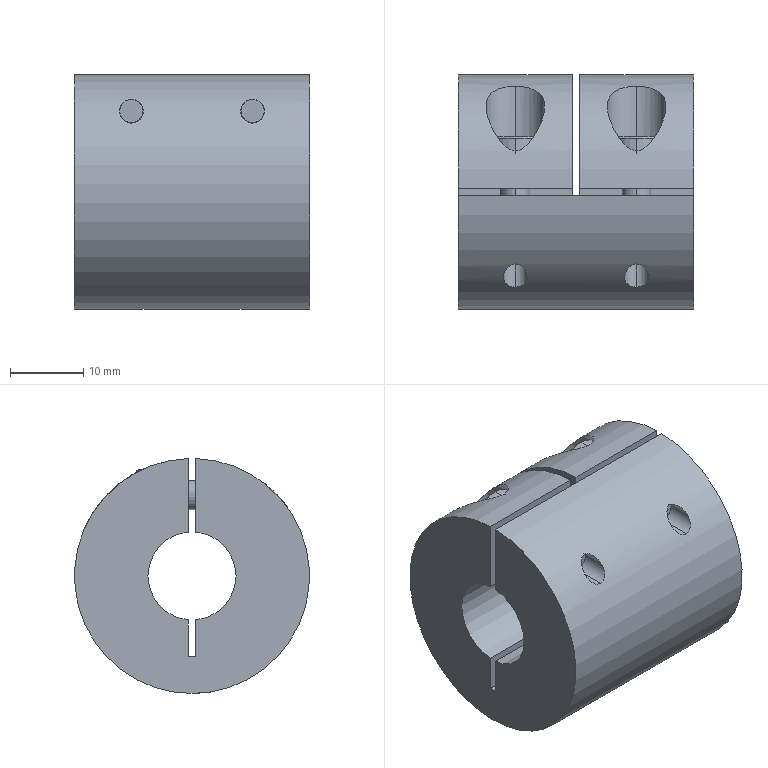Part | STEP file | coupling DCQ03-D32-d12-e14 | 3 solids | 70 faces | box 32 x 32 x 31.992 mm | volume 20201 mm3 | plane 35 | cylinder 27 | cone 8 | commonest cylinder face diameters 3.242 x4 4 x4 4.5 x4 7 x4 8 x4 32 x3